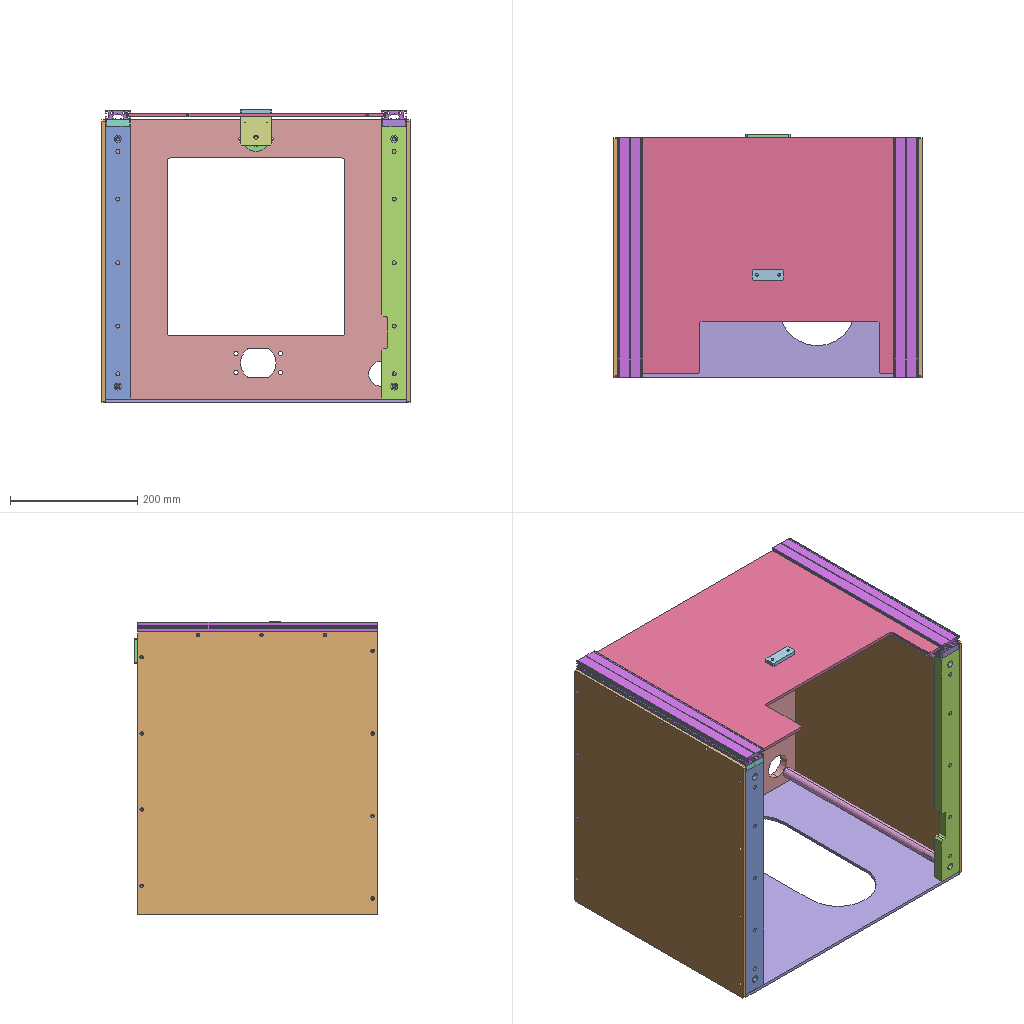Assembly | SolidWorks | 14 different items | 19 placed | box 485 x 382 x 461 mm
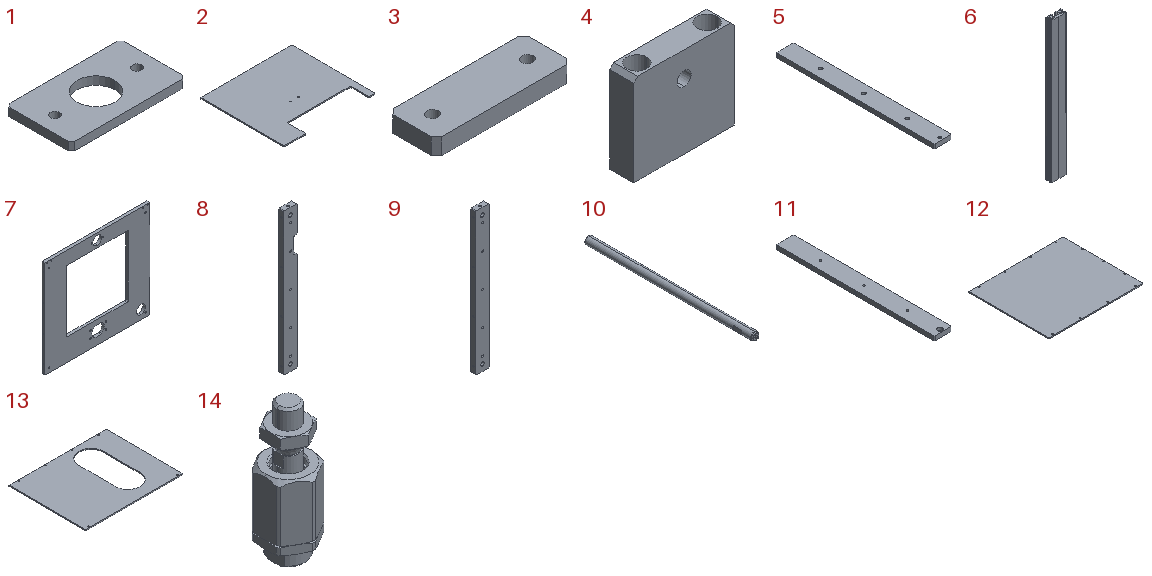Parts list (item | quantity | size | volume | features):
1 | x1 | 70 x 40 x 5 mm | 11645 mm3 | features Chamfer 1, FlatPattern 1, HoleWzd 1, ICE 1, SMBaseFlange 1, SheetMetal 1
2 | x1 | 406 x 372 x 5 mm | 637645 mm3 | features Extrusion 1, Fillet 1, HoleWzd 1, ICE 1
3 | x1 | 50 x 18 x 6 mm | 5186 mm3 | features Chamfer 1, Extrusion 1, HoleWzd 1
4 | x1 | 50 x 12 x 45 mm | 20517 mm3 | features HoleWzd 2, Chamfer 1, Extrusion 1
5 | x1 | 40 x 365 x 10 mm | 143435 mm3 | features MirrorStock 1
6 | x2 | 40 x 15 x 377 mm | 132086 mm3 | features BaseBody 1, MoveFace 1
7 | x1 | 475 x 12 x 440 mm | 1500689 mm3 | features HoleWzd 6, ICE 3, Fillet 2, Chamfer 1, Cut 1, Extrusion 1, MirrorPattern 1
8 | x1 | 40 x 15 x 430 mm | 242851 mm3 | features HoleWzd 6, Chamfer 2, ICE 2, Extrusion 1, Fillet 1
9 | x1 | 40 x 15 x 430 mm | 250428 mm3 | features HoleWzd 6, Chamfer 2, ICE 2, Extrusion 1, Fillet 1
10 | x4 | 16 x 353 x 16 mm | 69897 mm3 | features Chamfer 2, HoleWzd 2, ICE 2, Extrusion 1, MirrorPattern 1
11 | x1 | 40 x 365 x 10 mm | 143435 mm3 | features HoleWzd 4, Chamfer 1, Extrusion 1
12 | x2 | 445 x 377 x 5 mm | 837478 mm3 | features Extrusion 1, Fillet 1, HoleWzd 1
13 | x1 | 475 x 377 x 5 mm | 730114 mm3 | features Extrusion 1, HoleWzd 1, ICE 1
14 | x1 | 17 x 19 x 49 mm | 7093 mm3 | features BaseBody 7
Mates (type | each side: item.copy, entity, surface, feature):
Concentric | 9.1 face cylinder Cut-Extrude1 | 10.1 face cylinder Boss-Extrude1
Concentric | 9.1 face cylinder Cut-Extrude1 | 10.2 face cylinder Boss-Extrude1
Coincident | 7.1 face plane Boss-Extrude1 | 12.1 face plane Boss-Extrude1
Coincident | 7.1 face plane Boss-Extrude1 | 13.1 face plane Boss-Extrude1 | 3 times
Coincident | 7.1 face plane Boss-Extrude1 | 1.1 face plane Base-Flange1
Parallel | 7.1 face plane Boss-Extrude1 | 1.1 face plane Base-Flange1
Concentric | 7.1 face cylinder Cut-Extrude2 | 1.1 face cylinder Cut-Extrude1
Coincident | 11.1 face plane Boss-Extrude1 | 9.1 face plane Boss-Extrude1 | 3 times
Coincident | 11.1 face plane Boss-Extrude1 | 12.1 face plane Boss-Extrude1 | 2 times
Coincident | 11.1 face plane Boss-Extrude1 | 7.1 face plane Boss-Extrude1 | 3 times
Coincident | 9.1 face plane Boss-Extrude1 | 10.2 face plane Boss-Extrude1
Coincident | 10.1 face plane Boss-Extrude1 | 9.1 edge
Concentric | 2.1 face cylinder M5 Clearance Hole1 | 4.1 face cylinder Hex socket cap screw hole type 1 | 2 times
Coincident | 2.1 face plane Boss-Extrude1 | 4.1 face plane Boss-Extrude1
Parallel | 2.1 face plane Cut-Extrude1 | 4.1 face plane Boss-Extrude1
Concentric | 2.1 face cylinder M5 Clearance Hole1 | 3.1 face cylinder M5 Tapped Hole1 | 2 times
Coincident | 2.1 face plane Boss-Extrude1 | 3.1 face plane Boss-Extrude1
Coincident | 11.1 face plane Boss-Extrude1 | 6.1 face plane Input 1
Coincident | 12.1 face plane Boss-Extrude1 | 6.1 face plane Input 1
Coincident | 7.1 face plane Boss-Extrude1 | 6.1 face plane Input 1
Concentric | 8.1 face cylinder Cut-Extrude1 | 10.3 face cylinder Boss-Extrude2
Coincident | 8.1 face plane Boss-Extrude1 | 10.3 face plane Boss-Extrude1
Coincident | 7.1 face plane Boss-Extrude1 | 5.1 face plane 1-LST240520-OP10U02-1-P12_Mirror
Coincident | 12.2 face plane Boss-Extrude1 | 7.1 face plane Boss-Extrude1
Coincident | 8.1 face plane Boss-Extrude1 | 12.2 face plane Boss-Extrude1
Parallel | 8.1 face plane Boss-Extrude1 | 12.2 face plane Boss-Extrude1
Coincident | 11.1 face plane Boss-Extrude1 | 5.1 face plane 1-LST240520-OP10U02-1-P12_Mirror
Coincident | 12.2 face plane Boss-Extrude1 | 5.1 face plane 1-LST240520-OP10U02-1-P12_Mirror
Coincident | 8.1 face plane Boss-Extrude1 | 5.1 face plane 1-LST240520-OP10U02-1-P12_Mirror
Concentric | 8.1 face cylinder M6 Tapped Hole2 | 5.1 face cylinder 1-LST240520-OP10U02-1-P12_Mirror
Coincident | 6.2 face plane Input 1 | 6.1 face plane Input 1 | 2 times
Coincident | 12.2 face plane Boss-Extrude1 | 6.2 face plane Input 1
Width | 2.1 face plane Boss-Extrude1 | 2.1 face plane Boss-Extrude1 | 6.1 face plane Input 1 | 6.1 face plane Input 1
Width | 2.1 face plane Boss-Extrude1 | 2.1 face plane Boss-Extrude1 | 6.1 face plane Input 1 | 6.2 face plane Input 1
Concentric | 10.4 face cylinder Boss-Extrude2 | 8.1 face cylinder Hex socket cap screw hole type 1
Coincident | 10.4 face plane Boss-Extrude1 | 8.1 face plane Boss-Extrude1
Coincident | 12.1 face plane Boss-Extrude1 | 12.2 face plane Boss-Extrude1
Coincident | 4.1 face plane Boss-Extrude1 | 14.1 face plane _DIN-439-B - M8(F)-1-solid1